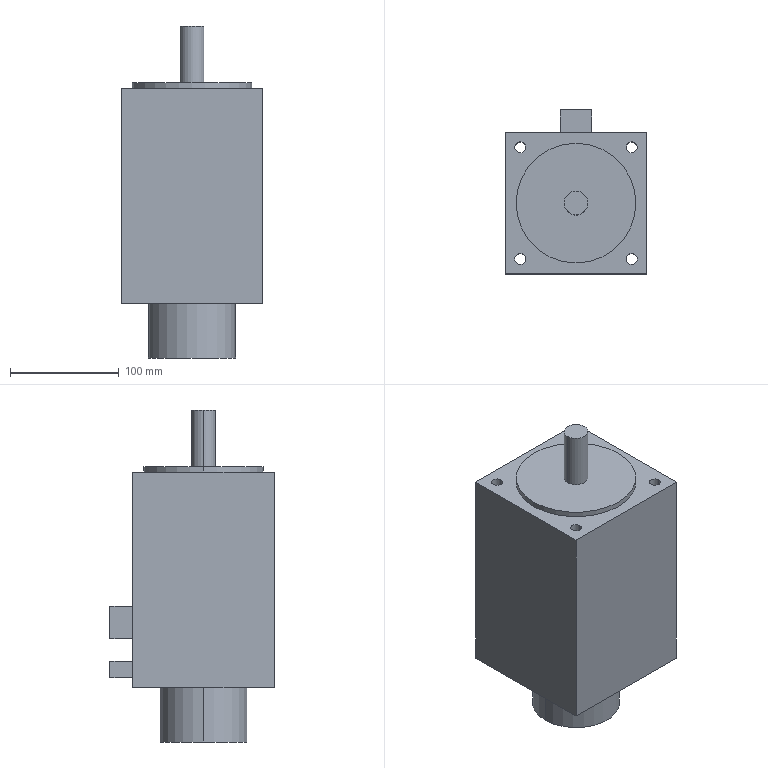Part | SolidWorks | features ICE 4, Extrusion 1 | 1 solid | 33 faces | box 130 x 151 x 305 mm | volume 3625077 mm3 | plane 19 | cylinder 14 | commonest cylinder face diameters 10 x8 22 x2 80 x2 110 x2
STEP:
#1=CARTESIAN_POINT('',(-40.,0.,-149.));
#2=VERTEX_POINT('',#1);
#3=CARTESIAN_POINT('',(40.,0.,-149.));
#4=VERTEX_POINT('',#3);
#5=CARTESIAN_POINT('',(0.,0.,-149.));
#6=DIRECTION('',(0.,0.,-1.));
#7=DIRECTION('',(-1.,0.,0.));
#8=AXIS2_PLACEMENT_3D('',#5,#6,#7);
#9=CIRCLE('',#8,40.);
#10=EDGE_CURVE('',#2,#4,#9,.T.);
#11=ORIENTED_EDGE('',*,*,#10,.F.);
#12=CARTESIAN_POINT('',(-40.,0.,-99.));
#13=VERTEX_POINT('',#12);
#14=CARTESIAN_POINT('',(-40.,0.,-149.));
#15=DIRECTION('',(0.,0.,1.));
#16=VECTOR('',#15,1000.);
#17=LINE('',#14,#16);
#18=EDGE_CURVE('',#2,#13,#17,.T.);
#19=ORIENTED_EDGE('',*,*,#18,.T.);
#20=CARTESIAN_POINT('',(40.,0.,-99.));
#21=VERTEX_POINT('',#20);
#22=CARTESIAN_POINT('',(0.,0.,-99.));
#23=DIRECTION('',(0.,0.,-1.));
#24=DIRECTION('',(1.,0.,0.));
#25=AXIS2_PLACEMENT_3D('',#22,#23,#24);
#26=CIRCLE('',#25,40.);
#27=EDGE_CURVE('',#13,#21,#26,.T.);
#28=ORIENTED_EDGE('',*,*,#27,.T.);
#29=CARTESIAN_POINT('',(40.,0.,-149.));
#30=DIRECTION('',(0.,0.,1.));
#31=VECTOR('',#30,1000.);
#32=LINE('',#29,#31);
#33=EDGE_CURVE('',#4,#21,#32,.T.);
#34=ORIENTED_EDGE('',*,*,#33,.F.);
#35=EDGE_LOOP('',(#11,#19,#28,#34));
#36=FACE_OUTER_BOUND('',#35,.T.);
#37=CARTESIAN_POINT('',(0.,0.,-149.));
#38=DIRECTION('',(0.,0.,1.));
#39=DIRECTION('',(1.,0.,0.));
#40=AXIS2_PLACEMENT_3D('',#37,#38,#39);
#41=CYLINDRICAL_SURFACE('',#40,40.);
#42=ADVANCED_FACE('',(#36),#41,.T.);
#43=CARTESIAN_POINT('',(11.,0.,156.));
#44=VERTEX_POINT('',#43);
#45=CARTESIAN_POINT('',(-11.,0.,156.));
#46=VERTEX_POINT('',#45);
#47=CARTESIAN_POINT('',(0.,0.,156.));
#48=DIRECTION('',(0.,0.,1.));
#49=DIRECTION('',(1.,0.,0.));
#50=AXIS2_PLACEMENT_3D('',#47,#48,#49);
#51=CIRCLE('',#50,11.);
#52=EDGE_CURVE('',#44,#46,#51,.T.);
#53=ORIENTED_EDGE('',*,*,#52,.F.);
#54=CARTESIAN_POINT('',(11.,0.,104.));
#55=VERTEX_POINT('',#54);
#56=CARTESIAN_POINT('',(11.,0.,156.));
#57=DIRECTION('',(0.,0.,-1.));
#58=VECTOR('',#57,1000.);
#59=LINE('',#56,#58);
#60=EDGE_CURVE('',#44,#55,#59,.T.);
#61=ORIENTED_EDGE('',*,*,#60,.T.);
#62=CARTESIAN_POINT('',(-11.,0.,104.));
#63=VERTEX_POINT('',#62);
#64=CARTESIAN_POINT('',(0.,0.,104.));
#65=DIRECTION('',(0.,0.,1.));
#66=DIRECTION('',(1.,0.,0.));
#67=AXIS2_PLACEMENT_3D('',#64,#65,#66);
#68=CIRCLE('',#67,11.);
#69=EDGE_CURVE('',#55,#63,#68,.T.);
#70=ORIENTED_EDGE('',*,*,#69,.T.);
#71=CARTESIAN_POINT('',(-11.,0.,156.));
#72=DIRECTION('',(0.,0.,-1.));
#73=VECTOR('',#72,1000.);
#74=LINE('',#71,#73);
#75=EDGE_CURVE('',#46,#63,#74,.T.);
#76=ORIENTED_EDGE('',*,*,#75,.F.);
#77=EDGE_LOOP('',(#53,#61,#70,#76));
#78=FACE_OUTER_BOUND('',#77,.T.);
#79=CARTESIAN_POINT('',(0.,0.,156.));
#80=DIRECTION('',(0.,0.,-1.));
#81=DIRECTION('',(-1.,0.,0.));
#82=AXIS2_PLACEMENT_3D('',#79,#80,#81);
#83=CYLINDRICAL_SURFACE('',#82,11.);
#84=ADVANCED_FACE('',(#78),#83,.T.);
#85=CARTESIAN_POINT('',(55.,0.,104.));
#86=VERTEX_POINT('',#85);
#87=CARTESIAN_POINT('',(-55.,0.,104.));
#88=VERTEX_POINT('',#87);
#89=CARTESIAN_POINT('',(0.,0.,104.));
#90=DIRECTION('',(0.,0.,1.));
#91=DIRECTION('',(1.,0.,0.));
#92=AXIS2_PLACEMENT_3D('',#89,#90,#91);
#93=CIRCLE('',#92,55.);
#94=EDGE_CURVE('',#86,#88,#93,.T.);
#95=ORIENTED_EDGE('',*,*,#94,.F.);
#96=CARTESIAN_POINT('',(55.,0.,99.));
#97=VERTEX_POINT('',#96);
#98=CARTESIAN_POINT('',(55.,0.,104.));
#99=DIRECTION('',(0.,0.,-1.));
#100=VECTOR('',#99,1000.);
#101=LINE('',#98,#100);
#102=EDGE_CURVE('',#86,#97,#101,.T.);
#103=ORIENTED_EDGE('',*,*,#102,.T.);
#104=CARTESIAN_POINT('',(-55.,0.,99.));
#105=VERTEX_POINT('',#104);
#106=CARTESIAN_POINT('',(0.,0.,99.));
#107=DIRECTION('',(0.,0.,1.));
#108=DIRECTION('',(1.,0.,0.));
#109=AXIS2_PLACEMENT_3D('',#106,#107,#108);
#110=CIRCLE('',#109,55.);
#111=EDGE_CURVE('',#97,#105,#110,.T.);
#112=ORIENTED_EDGE('',*,*,#111,.T.);
#113=CARTESIAN_POINT('',(-55.,0.,104.));
#114=DIRECTION('',(0.,0.,-1.));
#115=VECTOR('',#114,1000.);
#116=LINE('',#113,#115);
#117=EDGE_CURVE('',#88,#105,#116,.T.);
#118=ORIENTED_EDGE('',*,*,#117,.F.);
#119=EDGE_LOOP('',(#95,#103,#112,#118));
#120=FACE_OUTER_BOUND('',#119,.T.);
#121=CARTESIAN_POINT('',(0.,0.,104.));
#122=DIRECTION('',(0.,0.,-1.));
#123=DIRECTION('',(-1.,0.,0.));
#124=AXIS2_PLACEMENT_3D('',#121,#122,#123);
#125=CYLINDRICAL_SURFACE('',#124,55.);
#126=ADVANCED_FACE('',(#120),#125,.T.);
#127=CARTESIAN_POINT('',(46.265,-51.265,99.));
#128=VERTEX_POINT('',#127);
#129=CARTESIAN_POINT('',(56.265,-51.265,99.));
#130=VERTEX_POINT('',#129);
#131=CARTESIAN_POINT('',(51.265,-51.265,99.));
#132=DIRECTION('',(0.,0.,1.));
#133=DIRECTION('',(1.,0.,0.));
#134=AXIS2_PLACEMENT_3D('',#131,#132,#133);
#135=CIRCLE('',#134,5.);
#136=EDGE_CURVE('',#128,#130,#135,.T.);
#137=ORIENTED_EDGE('',*,*,#136,.T.);
#138=CARTESIAN_POINT('',(56.265,-51.265,-99.));
#139=VERTEX_POINT('',#138);
#140=CARTESIAN_POINT('',(56.265,-51.265,99.));
#141=DIRECTION('',(0.,0.,-1.));
#142=VECTOR('',#141,1000.);
#143=LINE('',#140,#142);
#144=EDGE_CURVE('',#130,#139,#143,.T.);
#145=ORIENTED_EDGE('',*,*,#144,.T.);
#146=CARTESIAN_POINT('',(46.265,-51.265,-99.));
#147=VERTEX_POINT('',#146);
#148=CARTESIAN_POINT('',(51.265,-51.265,-99.));
#149=DIRECTION('',(0.,0.,1.));
#150=DIRECTION('',(1.,0.,0.));
#151=AXIS2_PLACEMENT_3D('',#148,#149,#150);
#152=CIRCLE('',#151,5.);
#153=EDGE_CURVE('',#147,#139,#152,.T.);
#154=ORIENTED_EDGE('',*,*,#153,.F.);
#155=CARTESIAN_POINT('',(46.265,-51.265,99.));
#156=DIRECTION('',(0.,0.,-1.));
#157=VECTOR('',#156,1000.);
#158=LINE('',#155,#157);
#159=EDGE_CURVE('',#128,#147,#158,.T.);
#160=ORIENTED_EDGE('',*,*,#159,.F.);
#161=EDGE_LOOP('',(#137,#145,#154,#160));
#162=FACE_OUTER_BOUND('',#161,.T.);
#163=CARTESIAN_POINT('',(51.265,-51.265,99.));
#164=DIRECTION('',(0.,0.,-1.));
#165=DIRECTION('',(-1.,0.,0.));
#166=AXIS2_PLACEMENT_3D('',#163,#164,#165);
#167=CYLINDRICAL_SURFACE('',#166,5.);
#168=ADVANCED_FACE('',(#162),#167,.F.);
#169=CARTESIAN_POINT('',(-56.265,-51.265,99.));
#170=VERTEX_POINT('',#169);
#171=CARTESIAN_POINT('',(-46.265,-51.265,99.));
#172=VERTEX_POINT('',#171);
#173=CARTESIAN_POINT('',(-51.265,-51.265,99.));
#174=DIRECTION('',(0.,0.,1.));
#175=DIRECTION('',(-1.,0.,0.));
#176=AXIS2_PLACEMENT_3D('',#173,#174,#175);
#177=CIRCLE('',#176,5.);
#178=EDGE_CURVE('',#170,#172,#177,.T.);
#179=ORIENTED_EDGE('',*,*,#178,.T.);
#180=CARTESIAN_POINT('',(-46.265,-51.265,-99.));
#181=VERTEX_POINT('',#180);
#182=CARTESIAN_POINT('',(-46.265,-51.265,99.));
#183=DIRECTION('',(0.,0.,-1.));
#184=VECTOR('',#183,1000.);
#185=LINE('',#182,#184);
#186=EDGE_CURVE('',#172,#181,#185,.T.);
#187=ORIENTED_EDGE('',*,*,#186,.T.);
#188=CARTESIAN_POINT('',(-56.265,-51.265,-99.));
#189=VERTEX_POINT('',#188);
#190=CARTESIAN_POINT('',(-51.265,-51.265,-99.));
#191=DIRECTION('',(0.,0.,1.));
#192=DIRECTION('',(-1.,0.,0.));
#193=AXIS2_PLACEMENT_3D('',#190,#191,#192);
#194=CIRCLE('',#193,5.);
#195=EDGE_CURVE('',#189,#181,#194,.T.);
#196=ORIENTED_EDGE('',*,*,#195,.F.);
#197=CARTESIAN_POINT('',(-56.265,-51.265,99.));
#198=DIRECTION('',(0.,0.,-1.));
#199=VECTOR('',#198,1000.);
#200=LINE('',#197,#199);
#201=EDGE_CURVE('',#170,#189,#200,.T.);
#202=ORIENTED_EDGE('',*,*,#201,.F.);
#203=EDGE_LOOP('',(#179,#187,#196,#202));
#204=FACE_OUTER_BOUND('',#203,.T.);
#205=CARTESIAN_POINT('',(-51.265,-51.265,99.));
#206=DIRECTION('',(0.,0.,-1.));
#207=DIRECTION('',(-1.,0.,0.));
#208=AXIS2_PLACEMENT_3D('',#205,#206,#207);
#209=CYLINDRICAL_SURFACE('',#208,5.);
#210=ADVANCED_FACE('',(#204),#209,.F.);
#211=CARTESIAN_POINT('',(46.265,51.265,99.));
#212=VERTEX_POINT('',#211);
#213=CARTESIAN_POINT('',(56.265,51.265,99.));
#214=VERTEX_POINT('',#213);
#215=CARTESIAN_POINT('',(51.265,51.265,99.));
#216=DIRECTION('',(0.,0.,1.));
#217=DIRECTION('',(-1.,0.,0.));
#218=AXIS2_PLACEMENT_3D('',#215,#216,#217);
#219=CIRCLE('',#218,5.);
#220=EDGE_CURVE('',#212,#214,#219,.T.);
#221=ORIENTED_EDGE('',*,*,#220,.T.);
#222=CARTESIAN_POINT('',(56.265,51.265,-99.));
#223=VERTEX_POINT('',#222);
#224=CARTESIAN_POINT('',(56.265,51.265,99.));
#225=DIRECTION('',(0.,0.,-1.));
#226=VECTOR('',#225,1000.);
#227=LINE('',#224,#226);
#228=EDGE_CURVE('',#214,#223,#227,.T.);
#229=ORIENTED_EDGE('',*,*,#228,.T.);
#230=CARTESIAN_POINT('',(46.265,51.265,-99.));
#231=VERTEX_POINT('',#230);
#232=CARTESIAN_POINT('',(51.265,51.265,-99.));
#233=DIRECTION('',(0.,0.,1.));
#234=DIRECTION('',(-1.,0.,0.));
#235=AXIS2_PLACEMENT_3D('',#232,#233,#234);
#236=CIRCLE('',#235,5.);
#237=EDGE_CURVE('',#231,#223,#236,.T.);
#238=ORIENTED_EDGE('',*,*,#237,.F.);
#239=CARTESIAN_POINT('',(46.265,51.265,99.));
#240=DIRECTION('',(0.,0.,-1.));
#241=VECTOR('',#240,1000.);
#242=LINE('',#239,#241);
#243=EDGE_CURVE('',#212,#231,#242,.T.);
#244=ORIENTED_EDGE('',*,*,#243,.F.);
#245=EDGE_LOOP('',(#221,#229,#238,#244));
#246=FACE_OUTER_BOUND('',#245,.T.);
#247=CARTESIAN_POINT('',(51.265,51.265,99.));
#248=DIRECTION('',(0.,0.,-1.));
#249=DIRECTION('',(-1.,0.,0.));
#250=AXIS2_PLACEMENT_3D('',#247,#248,#249);
#251=CYLINDRICAL_SURFACE('',#250,5.);
#252=ADVANCED_FACE('',(#246),#251,.F.);
#253=CARTESIAN_POINT('',(-56.265,51.265,99.));
#254=VERTEX_POINT('',#253);
#255=CARTESIAN_POINT('',(-46.265,51.265,99.));
#256=VERTEX_POINT('',#255);
#257=CARTESIAN_POINT('',(-51.265,51.265,99.));
#258=DIRECTION('',(0.,0.,1.));
#259=DIRECTION('',(1.,0.,0.));
#260=AXIS2_PLACEMENT_3D('',#257,#258,#259);
#261=CIRCLE('',#260,5.);
#262=EDGE_CURVE('',#254,#256,#261,.T.);
#263=ORIENTED_EDGE('',*,*,#262,.T.);
#264=CARTESIAN_POINT('',(-46.265,51.265,-99.));
#265=VERTEX_POINT('',#264);
#266=CARTESIAN_POINT('',(-46.265,51.265,99.));
#267=DIRECTION('',(0.,0.,-1.));
#268=VECTOR('',#267,1000.);
#269=LINE('',#266,#268);
#270=EDGE_CURVE('',#256,#265,#269,.T.);
#271=ORIENTED_EDGE('',*,*,#270,.T.);
#272=CARTESIAN_POINT('',(-56.265,51.265,-99.));
#273=VERTEX_POINT('',#272);
#274=CARTESIAN_POINT('',(-51.265,51.265,-99.));
#275=DIRECTION('',(0.,0.,1.));
#276=DIRECTION('',(1.,0.,0.));
#277=AXIS2_PLACEMENT_3D('',#274,#275,#276);
#278=CIRCLE('',#277,5.);
#279=EDGE_CURVE('',#273,#265,#278,.T.);
#280=ORIENTED_EDGE('',*,*,#279,.F.);
#281=CARTESIAN_POINT('',(-56.265,51.265,99.));
#282=DIRECTION('',(0.,0.,-1.));
#283=VECTOR('',#282,1000.);
#284=LINE('',#281,#283);
#285=EDGE_CURVE('',#254,#273,#284,.T.);
#286=ORIENTED_EDGE('',*,*,#285,.F.);
#287=EDGE_LOOP('',(#263,#271,#280,#286));
#288=FACE_OUTER_BOUND('',#287,.T.);
#289=CARTESIAN_POINT('',(-51.265,51.265,99.));
#290=DIRECTION('',(0.,0.,-1.));
#291=DIRECTION('',(-1.,0.,0.));
#292=AXIS2_PLACEMENT_3D('',#289,#290,#291);
#293=CYLINDRICAL_SURFACE('',#292,5.);
#294=ADVANCED_FACE('',(#288),#293,.F.);
#295=CARTESIAN_POINT('',(-14.292,65.,-54.243));
#296=VERTEX_POINT('',#295);
#297=CARTESIAN_POINT('',(-14.292,65.,-24.297));
#298=VERTEX_POINT('',#297);
#299=CARTESIAN_POINT('',(-14.292,65.,99.));
#300=DIRECTION('',(0.,0.,1.));
#301=VECTOR('',#300,1000.);
#302=LINE('',#299,#301);
#303=EDGE_CURVE('',#296,#298,#302,.T.);
#304=ORIENTED_EDGE('',*,*,#303,.F.);
#305=CARTESIAN_POINT('',(14.292,65.,-54.243));
#306=VERTEX_POINT('',#305);
#307=CARTESIAN_POINT('',(-65.,65.,-54.243));
#308=DIRECTION('',(-1.,0.,0.));
#309=VECTOR('',#308,1000.);
#310=LINE('',#307,#309);
#311=EDGE_CURVE('',#306,#296,#310,.T.);
#312=ORIENTED_EDGE('',*,*,#311,.F.);
#313=CARTESIAN_POINT('',(14.292,65.,-24.297));
#314=VERTEX_POINT('',#313);
#315=CARTESIAN_POINT('',(14.292,65.,99.));
#316=DIRECTION('',(0.,0.,-1.));
#317=VECTOR('',#316,1000.);
#318=LINE('',#315,#317);
#319=EDGE_CURVE('',#314,#306,#318,.T.);
#320=ORIENTED_EDGE('',*,*,#319,.F.);
#321=CARTESIAN_POINT('',(-65.,65.,-24.297));
#322=DIRECTION('',(1.,0.,0.));
#323=VECTOR('',#322,1000.);
#324=LINE('',#321,#323);
#325=EDGE_CURVE('',#298,#314,#324,.T.);
#326=ORIENTED_EDGE('',*,*,#325,.F.);
#327=EDGE_LOOP('',(#304,#312,#320,#326));
#328=FACE_BOUND('',#327,.T.);
#329=CARTESIAN_POINT('',(65.,65.,-99.));
#330=VERTEX_POINT('',#329);
#331=CARTESIAN_POINT('',(-65.,65.,-99.));
#332=VERTEX_POINT('',#331);
#333=CARTESIAN_POINT('',(-65.,65.,-99.));
#334=DIRECTION('',(-1.,0.,0.));
#335=VECTOR('',#334,1000.);
#336=LINE('',#333,#335);
#337=EDGE_CURVE('',#330,#332,#336,.T.);
#338=ORIENTED_EDGE('',*,*,#337,.T.);
#339=CARTESIAN_POINT('',(-65.,65.,99.));
#340=VERTEX_POINT('',#339);
#341=CARTESIAN_POINT('',(-65.,65.,99.));
#342=DIRECTION('',(0.,0.,-1.));
#343=VECTOR('',#342,1000.);
#344=LINE('',#341,#343);
#345=EDGE_CURVE('',#340,#332,#344,.T.);
#346=ORIENTED_EDGE('',*,*,#345,.F.);
#347=CARTESIAN_POINT('',(65.,65.,99.));
#348=VERTEX_POINT('',#347);
#349=CARTESIAN_POINT('',(-65.,65.,99.));
#350=DIRECTION('',(-1.,0.,0.));
#351=VECTOR('',#350,1000.);
#352=LINE('',#349,#351);
#353=EDGE_CURVE('',#348,#340,#352,.T.);
#354=ORIENTED_EDGE('',*,*,#353,.F.);
#355=CARTESIAN_POINT('',(65.,65.,99.));
#356=DIRECTION('',(0.,0.,-1.));
#357=VECTOR('',#356,1000.);
#358=LINE('',#355,#357);
#359=EDGE_CURVE('',#348,#330,#358,.T.);
#360=ORIENTED_EDGE('',*,*,#359,.T.);
#361=EDGE_LOOP('',(#338,#346,#354,#360));
#362=FACE_OUTER_BOUND('',#361,.T.);
#363=CARTESIAN_POINT('',(-7.146,65.,-89.973));
#364=VERTEX_POINT('',#363);
#365=CARTESIAN_POINT('',(-7.146,65.,-75.));
#366=VERTEX_POINT('',#365);
#367=CARTESIAN_POINT('',(-7.146,65.,99.));
#368=DIRECTION('',(0.,0.,1.));
#369=VECTOR('',#368,1000.);
#370=LINE('',#367,#369);
#371=EDGE_CURVE('',#364,#366,#370,.T.);
#372=ORIENTED_EDGE('',*,*,#371,.F.);
#373=CARTESIAN_POINT('',(7.146,65.,-89.973));
#374=VERTEX_POINT('',#373);
#375=CARTESIAN_POINT('',(-65.,65.,-89.973));
#376=DIRECTION('',(-1.,0.,0.));
#377=VECTOR('',#376,1000.);
#378=LINE('',#375,#377);
#379=EDGE_CURVE('',#374,#364,#378,.T.);
#380=ORIENTED_EDGE('',*,*,#379,.F.);
#381=CARTESIAN_POINT('',(7.146,65.,-75.));
#382=VERTEX_POINT('',#381);
#383=CARTESIAN_POINT('',(7.146,65.,99.));
#384=DIRECTION('',(0.,0.,-1.));
#385=VECTOR('',#384,1000.);
#386=LINE('',#383,#385);
#387=EDGE_CURVE('',#382,#374,#386,.T.);
#388=ORIENTED_EDGE('',*,*,#387,.F.);
#389=CARTESIAN_POINT('',(-65.,65.,-75.));
#390=DIRECTION('',(1.,0.,0.));
#391=VECTOR('',#390,1000.);
#392=LINE('',#389,#391);
#393=EDGE_CURVE('',#366,#382,#392,.T.);
#394=ORIENTED_EDGE('',*,*,#393,.F.);
#395=EDGE_LOOP('',(#372,#380,#388,#394));
#396=FACE_BOUND('',#395,.T.);
#397=CARTESIAN_POINT('',(-65.,65.,99.));
#398=DIRECTION('',(0.,-1.,0.));
#399=DIRECTION('',(0.,0.,-1.));
#400=AXIS2_PLACEMENT_3D('',#397,#398,#399);
#401=PLANE('',#400);
#402=ADVANCED_FACE('',(#328,#362,#396),#401,.F.);
#403=CARTESIAN_POINT('',(0.,0.,99.));
#404=DIRECTION('',(0.,0.,1.));
#405=DIRECTION('',(1.,0.,0.));
#406=AXIS2_PLACEMENT_3D('',#403,#404,#405);
#407=CIRCLE('',#406,55.);
#408=EDGE_CURVE('',#105,#97,#407,.T.);
#409=ORIENTED_EDGE('',*,*,#408,.F.);
#410=ORIENTED_EDGE('',*,*,#111,.F.);
#411=EDGE_LOOP('',(#409,#410));
#412=FACE_BOUND('',#411,.T.);
#413=ORIENTED_EDGE('',*,*,#178,.F.);
#414=CARTESIAN_POINT('',(-51.265,-51.265,99.));
#415=DIRECTION('',(0.,0.,1.));
#416=DIRECTION('',(-1.,0.,0.));
#417=AXIS2_PLACEMENT_3D('',#414,#415,#416);
#418=CIRCLE('',#417,5.);
#419=EDGE_CURVE('',#172,#170,#418,.T.);
#420=ORIENTED_EDGE('',*,*,#419,.F.);
#421=EDGE_LOOP('',(#413,#420));
#422=FACE_BOUND('',#421,.T.);
#423=ORIENTED_EDGE('',*,*,#262,.F.);
#424=CARTESIAN_POINT('',(-51.265,51.265,99.));
#425=DIRECTION('',(0.,0.,1.));
#426=DIRECTION('',(1.,0.,0.));
#427=AXIS2_PLACEMENT_3D('',#424,#425,#426);
#428=CIRCLE('',#427,5.);
#429=EDGE_CURVE('',#256,#254,#428,.T.);
#430=ORIENTED_EDGE('',*,*,#429,.F.);
#431=EDGE_LOOP('',(#423,#430));
#432=FACE_BOUND('',#431,.T.);
#433=CARTESIAN_POINT('',(-65.,-65.,99.));
#434=VERTEX_POINT('',#433);
#435=CARTESIAN_POINT('',(-65.,65.,99.));
#436=DIRECTION('',(0.,-1.,0.));
#437=VECTOR('',#436,1000.);
#438=LINE('',#435,#437);
#439=EDGE_CURVE('',#340,#434,#438,.T.);
#440=ORIENTED_EDGE('',*,*,#439,.T.);
#441=CARTESIAN_POINT('',(65.,-65.,99.));
#442=VERTEX_POINT('',#441);
#443=CARTESIAN_POINT('',(-65.,-65.,99.));
#444=DIRECTION('',(1.,0.,0.));
#445=VECTOR('',#444,1000.);
#446=LINE('',#443,#445);
#447=EDGE_CURVE('',#434,#442,#446,.T.);
#448=ORIENTED_EDGE('',*,*,#447,.T.);
#449=CARTESIAN_POINT('',(65.,65.,99.));
#450=DIRECTION('',(0.,1.,0.));
#451=VECTOR('',#450,1000.);
#452=LINE('',#449,#451);
#453=EDGE_CURVE('',#442,#348,#452,.T.);
#454=ORIENTED_EDGE('',*,*,#453,.T.);
#455=ORIENTED_EDGE('',*,*,#353,.T.);
#456=EDGE_LOOP('',(#440,#448,#454,#455));
#457=FACE_OUTER_BOUND('',#456,.T.);
#458=ORIENTED_EDGE('',*,*,#220,.F.);
#459=CARTESIAN_POINT('',(51.265,51.265,99.));
#460=DIRECTION('',(0.,0.,1.));
#461=DIRECTION('',(-1.,0.,0.));
#462=AXIS2_PLACEMENT_3D('',#459,#460,#461);
#463=CIRCLE('',#462,5.);
#464=EDGE_CURVE('',#214,#212,#463,.T.);
#465=ORIENTED_EDGE('',*,*,#464,.F.);
#466=EDGE_LOOP('',(#458,#465));
#467=FACE_BOUND('',#466,.T.);
#468=ORIENTED_EDGE('',*,*,#136,.F.);
#469=CARTESIAN_POINT('',(51.265,-51.265,99.));
#470=DIRECTION('',(0.,0.,1.));
#471=DIRECTION('',(1.,0.,0.));
#472=AXIS2_PLACEMENT_3D('',#469,#470,#471);
#473=CIRCLE('',#472,5.);
#474=EDGE_CURVE('',#130,#128,#473,.T.);
#475=ORIENTED_EDGE('',*,*,#474,.F.);
#476=EDGE_LOOP('',(#468,#475));
#477=FACE_BOUND('',#476,.T.);
#478=CARTESIAN_POINT('',(0.,0.,99.));
#479=DIRECTION('',(0.,0.,1.));
#480=DIRECTION('',(1.,0.,0.));
#481=AXIS2_PLACEMENT_3D('',#478,#479,#480);
#482=PLANE('',#481);
#483=ADVANCED_FACE('',(#412,#422,#432,#457,#467,#477),#482,.T.);
#484=CARTESIAN_POINT('',(0.,0.,-99.));
#485=DIRECTION('',(0.,0.,-1.));
#486=DIRECTION('',(1.,0.,0.));
#487=AXIS2_PLACEMENT_3D('',#484,#485,#486);
#488=CIRCLE('',#487,40.);
#489=EDGE_CURVE('',#21,#13,#488,.T.);
#490=ORIENTED_EDGE('',*,*,#489,.F.);
#491=ORIENTED_EDGE('',*,*,#27,.F.);
#492=EDGE_LOOP('',(#490,#491));
#493=FACE_BOUND('',#492,.T.);
#494=CARTESIAN_POINT('',(-65.,-65.,-99.));
#495=VERTEX_POINT('',#494);
#496=CARTESIAN_POINT('',(-65.,65.,-99.));
#497=DIRECTION('',(0.,-1.,0.));
#498=VECTOR('',#497,1000.);
#499=LINE('',#496,#498);
#500=EDGE_CURVE('',#332,#495,#499,.T.);
#501=ORIENTED_EDGE('',*,*,#500,.F.);
#502=ORIENTED_EDGE('',*,*,#337,.F.);
#503=CARTESIAN_POINT('',(65.,-65.,-99.));
#504=VERTEX_POINT('',#503);
#505=CARTESIAN_POINT('',(65.,65.,-99.));
#506=DIRECTION('',(0.,1.,0.));
#507=VECTOR('',#506,1000.);
#508=LINE('',#505,#507);
#509=EDGE_CURVE('',#504,#330,#508,.T.);
#510=ORIENTED_EDGE('',*,*,#509,.F.);
#511=CARTESIAN_POINT('',(-65.,-65.,-99.));
#512=DIRECTION('',(1.,0.,0.));
#513=VECTOR('',#512,1000.);
#514=LINE('',#511,#513);
#515=EDGE_CURVE('',#495,#504,#514,.T.);
#516=ORIENTED_EDGE('',*,*,#515,.F.);
#517=EDGE_LOOP('',(#501,#502,#510,#516));
#518=FACE_OUTER_BOUND('',#517,.T.);
#519=ORIENTED_EDGE('',*,*,#279,.T.);
#520=CARTESIAN_POINT('',(-51.265,51.265,-99.));
#521=DIRECTION('',(0.,0.,1.));
#522=DIRECTION('',(1.,0.,0.));
#523=AXIS2_PLACEMENT_3D('',#520,#521,#522);
#524=CIRCLE('',#523,5.);
#525=EDGE_CURVE('',#265,#273,#524,.T.);
#526=ORIENTED_EDGE('',*,*,#525,.T.);
#527=EDGE_LOOP('',(#519,#526));
#528=FACE_BOUND('',#527,.T.);
#529=ORIENTED_EDGE('',*,*,#237,.T.);
#530=CARTESIAN_POINT('',(51.265,51.265,-99.));
#531=DIRECTION('',(0.,0.,1.));
#532=DIRECTION('',(-1.,0.,0.));
#533=AXIS2_PLACEMENT_3D('',#530,#531,#532);
#534=CIRCLE('',#533,5.);
#535=EDGE_CURVE('',#223,#231,#534,.T.);
#536=ORIENTED_EDGE('',*,*,#535,.T.);
#537=EDGE_LOOP('',(#529,#536));
#538=FACE_BOUND('',#537,.T.);
#539=ORIENTED_EDGE('',*,*,#195,.T.);
#540=CARTESIAN_POINT('',(-51.265,-51.265,-99.));
#541=DIRECTION('',(0.,0.,1.));
#542=DIRECTION('',(-1.,0.,0.));
#543=AXIS2_PLACEMENT_3D('',#540,#541,#542);
#544=CIRCLE('',#543,5.);
#545=EDGE_CURVE('',#181,#189,#544,.T.);
#546=ORIENTED_EDGE('',*,*,#545,.T.);
#547=EDGE_LOOP('',(#539,#546));
#548=FACE_BOUND('',#547,.T.);
#549=ORIENTED_EDGE('',*,*,#153,.T.);
#550=CARTESIAN_POINT('',(51.265,-51.265,-99.));
#551=DIRECTION('',(0.,0.,1.));
#552=DIRECTION('',(1.,0.,0.));
#553=AXIS2_PLACEMENT_3D('',#550,#551,#552);
#554=CIRCLE('',#553,5.);
#555=EDGE_CURVE('',#139,#147,#554,.T.);
#556=ORIENTED_EDGE('',*,*,#555,.T.);
#557=EDGE_LOOP('',(#549,#556));
#558=FACE_BOUND('',#557,.T.);
#559=CARTESIAN_POINT('',(0.,0.,-99.));
#560=DIRECTION('',(0.,0.,1.));
#561=DIRECTION('',(1.,0.,0.));
#562=AXIS2_PLACEMENT_3D('',#559,#560,#561);
#563=PLANE('',#562);
#564=ADVANCED_FACE('',(#493,#518,#528,#538,#548,#558),#563,.F.);
#565=ORIENTED_EDGE('',*,*,#500,.T.);
#566=CARTESIAN_POINT('',(-65.,-65.,99.));
#567=DIRECTION('',(0.,0.,-1.));
#568=VECTOR('',#567,1000.);
#569=LINE('',#566,#568);
#570=EDGE_CURVE('',#434,#495,#569,.T.);
#571=ORIENTED_EDGE('',*,*,#570,.F.);
#572=ORIENTED_EDGE('',*,*,#439,.F.);
#573=ORIENTED_EDGE('',*,*,#345,.T.);
#574=EDGE_LOOP('',(#565,#571,#572,#573));
#575=FACE_OUTER_BOUND('',#574,.T.);
#576=CARTESIAN_POINT('',(-65.,65.,99.));
#577=DIRECTION('',(1.,0.,0.));
#578=DIRECTION('',(0.,1.,0.));
#579=AXIS2_PLACEMENT_3D('',#576,#577,#578);
#580=PLANE('',#579);
#581=ADVANCED_FACE('',(#575),#580,.F.);
#582=ORIENTED_EDGE('',*,*,#515,.T.);
#583=CARTESIAN_POINT('',(65.,-65.,99.));
#584=DIRECTION('',(0.,0.,-1.));
#585=VECTOR('',#584,1000.);
#586=LINE('',#583,#585);
#587=EDGE_CURVE('',#442,#504,#586,.T.);
#588=ORIENTED_EDGE('',*,*,#587,.F.);
#589=ORIENTED_EDGE('',*,*,#447,.F.);
#590=ORIENTED_EDGE('',*,*,#570,.T.);
#591=EDGE_LOOP('',(#582,#588,#589,#590));
#592=FACE_OUTER_BOUND('',#591,.T.);
#593=CARTESIAN_POINT('',(-65.,-65.,99.));
#594=DIRECTION('',(0.,1.,0.));
#595=DIRECTION('',(0.,0.,1.));
#596=AXIS2_PLACEMENT_3D('',#593,#594,#595);
#597=PLANE('',#596);
#598=ADVANCED_FACE('',(#592),#597,.F.);
#599=ORIENTED_EDGE('',*,*,#509,.T.);
#600=ORIENTED_EDGE('',*,*,#359,.F.);
#601=ORIENTED_EDGE('',*,*,#453,.F.);
#602=ORIENTED_EDGE('',*,*,#587,.T.);
#603=EDGE_LOOP('',(#599,#600,#601,#602));
#604=FACE_OUTER_BOUND('',#603,.T.);
#605=CARTESIAN_POINT('',(65.,65.,99.));
#606=DIRECTION('',(-1.,0.,0.));
#607=DIRECTION('',(0.,-1.,0.));
#608=AXIS2_PLACEMENT_3D('',#605,#606,#607);
#609=PLANE('',#608);
#610=ADVANCED_FACE('',(#604),#609,.F.);
#611=ORIENTED_EDGE('',*,*,#270,.F.);
#612=ORIENTED_EDGE('',*,*,#429,.T.);
#613=ORIENTED_EDGE('',*,*,#285,.T.);
#614=ORIENTED_EDGE('',*,*,#525,.F.);
#615=EDGE_LOOP('',(#611,#612,#613,#614));
#616=FACE_OUTER_BOUND('',#615,.T.);
#617=CARTESIAN_POINT('',(-51.265,51.265,99.));
#618=DIRECTION('',(0.,0.,-1.));
#619=DIRECTION('',(-1.,0.,0.));
#620=AXIS2_PLACEMENT_3D('',#617,#618,#619);
#621=CYLINDRICAL_SURFACE('',#620,5.);
#622=ADVANCED_FACE('',(#616),#621,.F.);
#623=ORIENTED_EDGE('',*,*,#228,.F.);
#624=ORIENTED_EDGE('',*,*,#464,.T.);
#625=ORIENTED_EDGE('',*,*,#243,.T.);
#626=ORIENTED_EDGE('',*,*,#535,.F.);
#627=EDGE_LOOP('',(#623,#624,#625,#626));
#628=FACE_OUTER_BOUND('',#627,.T.);
#629=CARTESIAN_POINT('',(51.265,51.265,99.));
#630=DIRECTION('',(0.,0.,-1.));
#631=DIRECTION('',(-1.,0.,0.));
#632=AXIS2_PLACEMENT_3D('',#629,#630,#631);
#633=CYLINDRICAL_SURFACE('',#632,5.);
#634=ADVANCED_FACE('',(#628),#633,.F.);
#635=ORIENTED_EDGE('',*,*,#186,.F.);
#636=ORIENTED_EDGE('',*,*,#419,.T.);
#637=ORIENTED_EDGE('',*,*,#201,.T.);
#638=ORIENTED_EDGE('',*,*,#545,.F.);
#639=EDGE_LOOP('',(#635,#636,#637,#638));
#640=FACE_OUTER_BOUND('',#639,.T.);
#641=CARTESIAN_POINT('',(-51.265,-51.265,99.));
#642=DIRECTION('',(0.,0.,-1.));
#643=DIRECTION('',(-1.,0.,0.));
#644=AXIS2_PLACEMENT_3D('',#641,#642,#643);
#645=CYLINDRICAL_SURFACE('',#644,5.);
#646=ADVANCED_FACE('',(#640),#645,.F.);
#647=ORIENTED_EDGE('',*,*,#144,.F.);
#648=ORIENTED_EDGE('',*,*,#474,.T.);
#649=ORIENTED_EDGE('',*,*,#159,.T.);
#650=ORIENTED_EDGE('',*,*,#555,.F.);
#651=EDGE_LOOP('',(#647,#648,#649,#650));
#652=FACE_OUTER_BOUND('',#651,.T.);
#653=CARTESIAN_POINT('',(51.265,-51.265,99.));
#654=DIRECTION('',(0.,0.,-1.));
#655=DIRECTION('',(-1.,0.,0.));
#656=AXIS2_PLACEMENT_3D('',#653,#654,#655);
#657=CYLINDRICAL_SURFACE('',#656,5.);
#658=ADVANCED_FACE('',(#652),#657,.F.);
#659=ORIENTED_EDGE('',*,*,#102,.F.);
#660=CARTESIAN_POINT('',(0.,0.,104.));
#661=DIRECTION('',(0.,0.,1.));
#662=DIRECTION('',(1.,0.,0.));
#663=AXIS2_PLACEMENT_3D('',#660,#661,#662);
#664=CIRCLE('',#663,55.);
#665=EDGE_CURVE('',#88,#86,#664,.T.);
#666=ORIENTED_EDGE('',*,*,#665,.F.);
#667=ORIENTED_EDGE('',*,*,#117,.T.);
#668=ORIENTED_EDGE('',*,*,#408,.T.);
#669=EDGE_LOOP('',(#659,#666,#667,#668));
#670=FACE_OUTER_BOUND('',#669,.T.);
#671=CARTESIAN_POINT('',(0.,0.,104.));
#672=DIRECTION('',(0.,0.,-1.));
#673=DIRECTION('',(-1.,0.,0.));
#674=AXIS2_PLACEMENT_3D('',#671,#672,#673);
#675=CYLINDRICAL_SURFACE('',#674,55.);
#676=ADVANCED_FACE('',(#670),#675,.T.);
#677=CARTESIAN_POINT('',(0.,0.,104.));
#678=DIRECTION('',(0.,0.,1.));
#679=DIRECTION('',(1.,0.,0.));
#680=AXIS2_PLACEMENT_3D('',#677,#678,#679);
#681=CIRCLE('',#680,11.);
#682=EDGE_CURVE('',#63,#55,#681,.T.);
#683=ORIENTED_EDGE('',*,*,#682,.F.);
#684=ORIENTED_EDGE('',*,*,#69,.F.);
#685=EDGE_LOOP('',(#683,#684));
#686=FACE_BOUND('',#685,.T.);
#687=ORIENTED_EDGE('',*,*,#665,.T.);
#688=ORIENTED_EDGE('',*,*,#94,.T.);
#689=EDGE_LOOP('',(#687,#688));
#690=FACE_OUTER_BOUND('',#689,.T.);
#691=CARTESIAN_POINT('',(0.,0.,104.));
#692=DIRECTION('',(0.,0.,1.));
#693=DIRECTION('',(1.,0.,0.));
#694=AXIS2_PLACEMENT_3D('',#691,#692,#693);
#695=PLANE('',#694);
#696=ADVANCED_FACE('',(#686,#690),#695,.T.);
#697=ORIENTED_EDGE('',*,*,#60,.F.);
#698=CARTESIAN_POINT('',(0.,0.,156.));
#699=DIRECTION('',(0.,0.,1.));
#700=DIRECTION('',(1.,0.,0.));
#701=AXIS2_PLACEMENT_3D('',#698,#699,#700);
#702=CIRCLE('',#701,11.);
#703=EDGE_CURVE('',#46,#44,#702,.T.);
#704=ORIENTED_EDGE('',*,*,#703,.F.);
#705=ORIENTED_EDGE('',*,*,#75,.T.);
#706=ORIENTED_EDGE('',*,*,#682,.T.);
#707=EDGE_LOOP('',(#697,#704,#705,#706));
#708=FACE_OUTER_BOUND('',#707,.T.);
#709=CARTESIAN_POINT('',(0.,0.,156.));
#710=DIRECTION('',(0.,0.,-1.));
#711=DIRECTION('',(-1.,0.,0.));
#712=AXIS2_PLACEMENT_3D('',#709,#710,#711);
#713=CYLINDRICAL_SURFACE('',#712,11.);
#714=ADVANCED_FACE('',(#708),#713,.T.);
#715=ORIENTED_EDGE('',*,*,#703,.T.);
#716=ORIENTED_EDGE('',*,*,#52,.T.);
#717=EDGE_LOOP('',(#715,#716));
#718=FACE_OUTER_BOUND('',#717,.T.);
#719=CARTESIAN_POINT('',(0.,0.,156.));
#720=DIRECTION('',(0.,0.,1.));
#721=DIRECTION('',(1.,0.,0.));
#722=AXIS2_PLACEMENT_3D('',#719,#720,#721);
#723=PLANE('',#722);
#724=ADVANCED_FACE('',(#718),#723,.T.);
#725=CARTESIAN_POINT('',(-14.292,86.,-54.243));
#726=VERTEX_POINT('',#725);
#727=CARTESIAN_POINT('',(-14.292,86.,-54.243));
#728=DIRECTION('',(0.,-1.,0.));
#729=VECTOR('',#728,1000.);
#730=LINE('',#727,#729);
#731=EDGE_CURVE('',#726,#296,#730,.T.);
#732=ORIENTED_EDGE('',*,*,#731,.T.);
#733=ORIENTED_EDGE('',*,*,#303,.T.);
#734=CARTESIAN_POINT('',(-14.292,86.,-24.297));
#735=VERTEX_POINT('',#734);
#736=CARTESIAN_POINT('',(-14.292,86.,-24.297));
#737=DIRECTION('',(0.,-1.,0.));
#738=VECTOR('',#737,1000.);
#739=LINE('',#736,#738);
#740=EDGE_CURVE('',#735,#298,#739,.T.);
#741=ORIENTED_EDGE('',*,*,#740,.F.);
#742=CARTESIAN_POINT('',(-14.292,86.,-24.297));
#743=DIRECTION('',(0.,0.,1.));
#744=VECTOR('',#743,1000.);
#745=LINE('',#742,#744);
#746=EDGE_CURVE('',#726,#735,#745,.T.);
#747=ORIENTED_EDGE('',*,*,#746,.F.);
#748=EDGE_LOOP('',(#732,#733,#741,#747));
#749=FACE_OUTER_BOUND('',#748,.T.);
#750=CARTESIAN_POINT('',(-14.292,86.,-24.297));
#751=DIRECTION('',(1.,0.,0.));
#752=DIRECTION('',(0.,0.,-1.));
#753=AXIS2_PLACEMENT_3D('',#750,#751,#752);
#754=PLANE('',#753);
#755=ADVANCED_FACE('',(#749),#754,.F.);
#756=ORIENTED_EDGE('',*,*,#740,.T.);
#757=ORIENTED_EDGE('',*,*,#325,.T.);
#758=CARTESIAN_POINT('',(14.292,86.,-24.297));
#759=VERTEX_POINT('',#758);
#760=CARTESIAN_POINT('',(14.292,86.,-24.297));
#761=DIRECTION('',(0.,-1.,0.));
#762=VECTOR('',#761,1000.);
#763=LINE('',#760,#762);
#764=EDGE_CURVE('',#759,#314,#763,.T.);
#765=ORIENTED_EDGE('',*,*,#764,.F.);
#766=CARTESIAN_POINT('',(14.292,86.,-24.297));
#767=DIRECTION('',(1.,0.,0.));
#768=VECTOR('',#767,1000.);
#769=LINE('',#766,#768);
#770=EDGE_CURVE('',#735,#759,#769,.T.);
#771=ORIENTED_EDGE('',*,*,#770,.F.);
#772=EDGE_LOOP('',(#756,#757,#765,#771));
#773=FACE_OUTER_BOUND('',#772,.T.);
#774=CARTESIAN_POINT('',(14.292,86.,-24.297));
#775=DIRECTION('',(0.,0.,-1.));
#776=DIRECTION('',(-1.,0.,0.));
#777=AXIS2_PLACEMENT_3D('',#774,#775,#776);
#778=PLANE('',#777);
#779=ADVANCED_FACE('',(#773),#778,.F.);
#780=ORIENTED_EDGE('',*,*,#764,.T.);
#781=ORIENTED_EDGE('',*,*,#319,.T.);
#782=CARTESIAN_POINT('',(14.292,86.,-54.243));
#783=VERTEX_POINT('',#782);
#784=CARTESIAN_POINT('',(14.292,86.,-54.243));
#785=DIRECTION('',(0.,-1.,0.));
#786=VECTOR('',#785,1000.);
#787=LINE('',#784,#786);
#788=EDGE_CURVE('',#783,#306,#787,.T.);
#789=ORIENTED_EDGE('',*,*,#788,.F.);
#790=CARTESIAN_POINT('',(14.292,86.,-24.297));
#791=DIRECTION('',(0.,0.,-1.));
#792=VECTOR('',#791,1000.);
#793=LINE('',#790,#792);
#794=EDGE_CURVE('',#759,#783,#793,.T.);
#795=ORIENTED_EDGE('',*,*,#794,.F.);
#796=EDGE_LOOP('',(#780,#781,#789,#795));
#797=FACE_OUTER_BOUND('',#796,.T.);
#798=CARTESIAN_POINT('',(14.292,86.,-24.297));
#799=DIRECTION('',(-1.,0.,0.));
#800=DIRECTION('',(0.,0.,1.));
#801=AXIS2_PLACEMENT_3D('',#798,#799,#800);
#802=PLANE('',#801);
#803=ADVANCED_FACE('',(#797),#802,.F.);
#804=ORIENTED_EDGE('',*,*,#788,.T.);
#805=ORIENTED_EDGE('',*,*,#311,.T.);
#806=ORIENTED_EDGE('',*,*,#731,.F.);
#807=CARTESIAN_POINT('',(14.292,86.,-54.243));
#808=DIRECTION('',(-1.,0.,0.));
#809=VECTOR('',#808,1000.);
#810=LINE('',#807,#809);
#811=EDGE_CURVE('',#783,#726,#810,.T.);
#812=ORIENTED_EDGE('',*,*,#811,.F.);
#813=EDGE_LOOP('',(#804,#805,#806,#812));
#814=FACE_OUTER_BOUND('',#813,.T.);
#815=CARTESIAN_POINT('',(14.292,86.,-54.243));
#816=DIRECTION('',(0.,0.,1.));
#817=DIRECTION('',(1.,0.,0.));
#818=AXIS2_PLACEMENT_3D('',#815,#816,#817);
#819=PLANE('',#818);
#820=ADVANCED_FACE('',(#814),#819,.F.);
#821=ORIENTED_EDGE('',*,*,#746,.T.);
#822=ORIENTED_EDGE('',*,*,#770,.T.);
#823=ORIENTED_EDGE('',*,*,#794,.T.);
#824=ORIENTED_EDGE('',*,*,#811,.T.);
#825=EDGE_LOOP('',(#821,#822,#823,#824));
#826=FACE_OUTER_BOUND('',#825,.T.);
#827=CARTESIAN_POINT('',(0.,86.,0.));
#828=DIRECTION('',(0.,1.,0.));
#829=DIRECTION('',(0.,0.,1.));
#830=AXIS2_PLACEMENT_3D('',#827,#828,#829);
#831=PLANE('',#830);
#832=ADVANCED_FACE('',(#826),#831,.T.);
#833=CARTESIAN_POINT('',(-7.146,86.,-89.973));
#834=VERTEX_POINT('',#833);
#835=CARTESIAN_POINT('',(-7.146,86.,-89.973));
#836=DIRECTION('',(0.,-1.,0.));
#837=VECTOR('',#836,1000.);
#838=LINE('',#835,#837);
#839=EDGE_CURVE('',#834,#364,#838,.T.);
#840=ORIENTED_EDGE('',*,*,#839,.T.);
#841=ORIENTED_EDGE('',*,*,#371,.T.);
#842=CARTESIAN_POINT('',(-7.146,86.,-75.));
#843=VERTEX_POINT('',#842);
#844=CARTESIAN_POINT('',(-7.146,86.,-75.));
#845=DIRECTION('',(0.,-1.,0.));
#846=VECTOR('',#845,1000.);
#847=LINE('',#844,#846);
#848=EDGE_CURVE('',#843,#366,#847,.T.);
#849=ORIENTED_EDGE('',*,*,#848,.F.);
#850=CARTESIAN_POINT('',(-7.146,86.,-75.));
#851=DIRECTION('',(0.,0.,1.));
#852=VECTOR('',#851,1000.);
#853=LINE('',#850,#852);
#854=EDGE_CURVE('',#834,#843,#853,.T.);
#855=ORIENTED_EDGE('',*,*,#854,.F.);
#856=EDGE_LOOP('',(#840,#841,#849,#855));
#857=FACE_OUTER_BOUND('',#856,.T.);
#858=CARTESIAN_POINT('',(-7.146,86.,-75.));
#859=DIRECTION('',(1.,0.,0.));
#860=DIRECTION('',(0.,0.,-1.));
#861=AXIS2_PLACEMENT_3D('',#858,#859,#860);
#862=PLANE('',#861);
#863=ADVANCED_FACE('',(#857),#862,.F.);
#864=ORIENTED_EDGE('',*,*,#848,.T.);
#865=ORIENTED_EDGE('',*,*,#393,.T.);
#866=CARTESIAN_POINT('',(7.146,86.,-75.));
#867=VERTEX_POINT('',#866);
#868=CARTESIAN_POINT('',(7.146,86.,-75.));
#869=DIRECTION('',(0.,-1.,0.));
#870=VECTOR('',#869,1000.);
#871=LINE('',#868,#870);
#872=EDGE_CURVE('',#867,#382,#871,.T.);
#873=ORIENTED_EDGE('',*,*,#872,.F.);
#874=CARTESIAN_POINT('',(7.146,86.,-75.));
#875=DIRECTION('',(1.,0.,0.));
#876=VECTOR('',#875,1000.);
#877=LINE('',#874,#876);
#878=EDGE_CURVE('',#843,#867,#877,.T.);
#879=ORIENTED_EDGE('',*,*,#878,.F.);
#880=EDGE_LOOP('',(#864,#865,#873,#879));
#881=FACE_OUTER_BOUND('',#880,.T.);
#882=CARTESIAN_POINT('',(7.146,86.,-75.));
#883=DIRECTION('',(0.,0.,-1.));
#884=DIRECTION('',(-1.,0.,0.));
#885=AXIS2_PLACEMENT_3D('',#882,#883,#884);
#886=PLANE('',#885);
#887=ADVANCED_FACE('',(#881),#886,.F.);
#888=ORIENTED_EDGE('',*,*,#872,.T.);
#889=ORIENTED_EDGE('',*,*,#387,.T.);
#890=CARTESIAN_POINT('',(7.146,86.,-89.973));
#891=VERTEX_POINT('',#890);
#892=CARTESIAN_POINT('',(7.146,86.,-89.973));
#893=DIRECTION('',(0.,-1.,0.));
#894=VECTOR('',#893,1000.);
#895=LINE('',#892,#894);
#896=EDGE_CURVE('',#891,#374,#895,.T.);
#897=ORIENTED_EDGE('',*,*,#896,.F.);
#898=CARTESIAN_POINT('',(7.146,86.,-75.));
#899=DIRECTION('',(0.,0.,-1.));
#900=VECTOR('',#899,1000.);
#901=LINE('',#898,#900);
#902=EDGE_CURVE('',#867,#891,#901,.T.);
#903=ORIENTED_EDGE('',*,*,#902,.F.);
#904=EDGE_LOOP('',(#888,#889,#897,#903));
#905=FACE_OUTER_BOUND('',#904,.T.);
#906=CARTESIAN_POINT('',(7.146,86.,-75.));
#907=DIRECTION('',(-1.,0.,0.));
#908=DIRECTION('',(0.,0.,1.));
#909=AXIS2_PLACEMENT_3D('',#906,#907,#908);
#910=PLANE('',#909);
#911=ADVANCED_FACE('',(#905),#910,.F.);
#912=ORIENTED_EDGE('',*,*,#896,.T.);
#913=ORIENTED_EDGE('',*,*,#379,.T.);
#914=ORIENTED_EDGE('',*,*,#839,.F.);
#915=CARTESIAN_POINT('',(7.146,86.,-89.973));
#916=DIRECTION('',(-1.,0.,0.));
#917=VECTOR('',#916,1000.);
#918=LINE('',#915,#917);
#919=EDGE_CURVE('',#891,#834,#918,.T.);
#920=ORIENTED_EDGE('',*,*,#919,.F.);
#921=EDGE_LOOP('',(#912,#913,#914,#920));
#922=FACE_OUTER_BOUND('',#921,.T.);
#923=CARTESIAN_POINT('',(7.146,86.,-89.973));
#924=DIRECTION('',(0.,0.,1.));
#925=DIRECTION('',(1.,0.,0.));
#926=AXIS2_PLACEMENT_3D('',#923,#924,#925);
#927=PLANE('',#926);
#928=ADVANCED_FACE('',(#922),#927,.F.);
#929=ORIENTED_EDGE('',*,*,#854,.T.);
#930=ORIENTED_EDGE('',*,*,#878,.T.);
#931=ORIENTED_EDGE('',*,*,#902,.T.);
#932=ORIENTED_EDGE('',*,*,#919,.T.);
#933=EDGE_LOOP('',(#929,#930,#931,#932));
#934=FACE_OUTER_BOUND('',#933,.T.);
#935=CARTESIAN_POINT('',(0.,86.,0.));
#936=DIRECTION('',(0.,1.,0.));
#937=DIRECTION('',(0.,0.,1.));
#938=AXIS2_PLACEMENT_3D('',#935,#936,#937);
#939=PLANE('',#938);
#940=ADVANCED_FACE('',(#934),#939,.T.);
#941=ORIENTED_EDGE('',*,*,#18,.F.);
#942=CARTESIAN_POINT('',(0.,0.,-149.));
#943=DIRECTION('',(0.,0.,-1.));
#944=DIRECTION('',(-1.,0.,0.));
#945=AXIS2_PLACEMENT_3D('',#942,#943,#944);
#946=CIRCLE('',#945,40.);
#947=EDGE_CURVE('',#4,#2,#946,.T.);
#948=ORIENTED_EDGE('',*,*,#947,.F.);
#949=ORIENTED_EDGE('',*,*,#33,.T.);
#950=ORIENTED_EDGE('',*,*,#489,.T.);
#951=EDGE_LOOP('',(#941,#948,#949,#950));
#952=FACE_OUTER_BOUND('',#951,.T.);
#953=CARTESIAN_POINT('',(0.,0.,-149.));
#954=DIRECTION('',(0.,0.,1.));
#955=DIRECTION('',(1.,0.,0.));
#956=AXIS2_PLACEMENT_3D('',#953,#954,#955);
#957=CYLINDRICAL_SURFACE('',#956,40.);
#958=ADVANCED_FACE('',(#952),#957,.T.);
#959=ORIENTED_EDGE('',*,*,#947,.T.);
#960=ORIENTED_EDGE('',*,*,#10,.T.);
#961=EDGE_LOOP('',(#959,#960));
#962=FACE_OUTER_BOUND('',#961,.T.);
#963=CARTESIAN_POINT('',(0.,0.,-149.));
#964=DIRECTION('',(0.,0.,-1.));
#965=DIRECTION('',(-1.,0.,0.));
#966=AXIS2_PLACEMENT_3D('',#963,#964,#965);
#967=PLANE('',#966);
#968=ADVANCED_FACE('',(#962),#967,.T.);
#969=CLOSED_SHELL('',(#42,#84,#126,#168,#210,#252,#294,#402,#483,#564,#581,#598,#610,#622,#634,#646,#658,#676,#696,#714,#724,#755,#779,#803,#820,#832,#863,#887,#911,#928,#940,#958,#968));
#970=MANIFOLD_SOLID_BREP('',#969);
#971=CARTESIAN_POINT('',(0.,0.,0.));
#972=DIRECTION('',(0.,0.,1.));
#973=DIRECTION('',(1.,0.,0.));
#974=AXIS2_PLACEMENT_3D('',#971,#972,#973);
#975=(LENGTH_UNIT()NAMED_UNIT(*)SI_UNIT(.MILLI.,.METRE.));
#976=UNCERTAINTY_MEASURE_WITH_UNIT(LENGTH_MEASURE(0.00001),#975,'','');
#977=(NAMED_UNIT(*)PLANE_ANGLE_UNIT()SI_UNIT($,.RADIAN.));
#978=(NAMED_UNIT(*)SI_UNIT($,.STERADIAN.)SOLID_ANGLE_UNIT());
#979=(GEOMETRIC_REPRESENTATION_CONTEXT(3)GLOBAL_UNCERTAINTY_ASSIGNED_CONTEXT((#976))GLOBAL_UNIT_ASSIGNED_CONTEXT((#975,#977,#978))REPRESENTATION_CONTEXT('',''));
#980=ADVANCED_BREP_SHAPE_REPRESENTATION('',(#970,#974),#979);